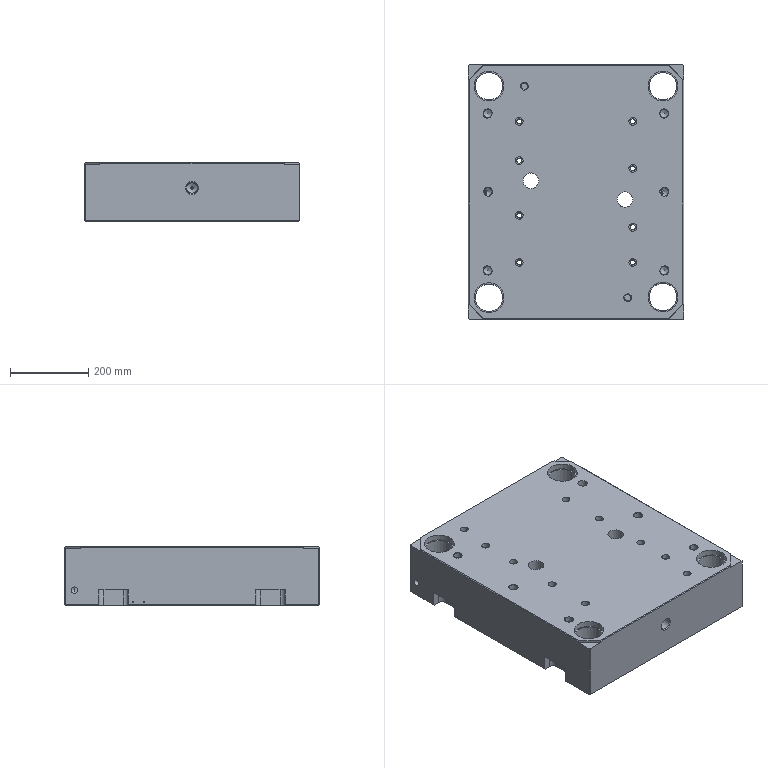Part | STEP file | P011002A001-000 | 1 solid | 1736 faces | box 550 x 650 x 150 mm | volume 35811112 mm3 | plane 923 | cone 276 | other 246 | cylinder 239 | spline 28 | sphere 16 | torus 8 | commonest cylinder face diameters 10 x51 6.8 x19 7.973 x19 8 x19 20 x18 24 x14